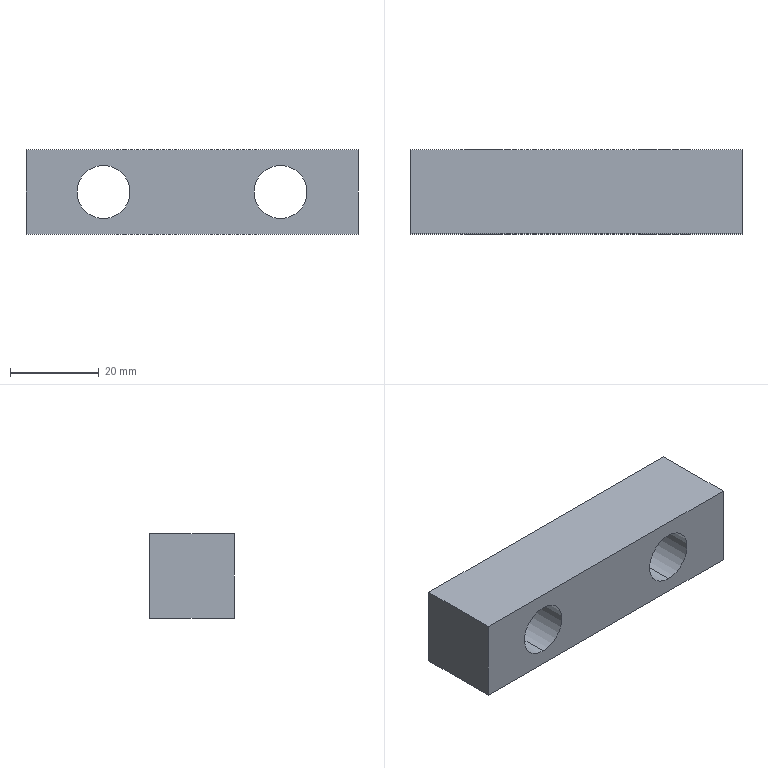Part | STEP file | [04]-1 | 1 solid | 10 faces | box 75 x 19 x 19 mm | volume 22777 mm3 | plane 6 | cylinder 4 | commonest cylinder face diameters 12 x4
STEP:
#1=CARTESIAN_POINT('',(0.,0.,0.));
#2=DIRECTION('',(0.,0.,1.));
#3=DIRECTION('',(1.,0.,0.));
#4=AXIS2_PLACEMENT_3D('',#1,#2,#3);
#5=CARTESIAN_POINT('',(17.5,-19.,15.5));
#6=VERTEX_POINT('',#5);
#7=CARTESIAN_POINT('',(17.5,0.,15.5));
#8=VERTEX_POINT('',#7);
#9=CARTESIAN_POINT('',(17.5,-19.,15.5));
#10=DIRECTION('',(0.,1.,0.));
#11=VECTOR('',#10,1.);
#12=LINE('',#9,#11);
#13=CARTESIAN_POINT('',(17.5,-19.,9.5));
#14=DIRECTION('',(0.,1.,0.));
#15=DIRECTION('',(0.,0.,1.));
#16=AXIS2_PLACEMENT_3D('',#13,#14,#15);
#17=CYLINDRICAL_SURFACE('',#16,6.);
#18=CARTESIAN_POINT('',(6.283,0.));
#19=DIRECTION('',(0.,1.));
#20=VECTOR('',#19,1.);
#21=LINE('',#18,#20);
#22=(GEOMETRIC_REPRESENTATION_CONTEXT(2)PARAMETRIC_REPRESENTATION_CONTEXT()REPRESENTATION_CONTEXT('',''));
#23=DEFINITIONAL_REPRESENTATION('',(#21),#22);
#24=PCURVE('',#17,#23);
#25=CARTESIAN_POINT('',(17.5,-19.,9.5));
#26=DIRECTION('',(0.,1.,0.));
#27=DIRECTION('',(0.,0.,1.));
#28=AXIS2_PLACEMENT_3D('',#25,#26,#27);
#29=CYLINDRICAL_SURFACE('',#28,6.);
#30=CARTESIAN_POINT('',(0.,0.));
#31=DIRECTION('',(0.,1.));
#32=VECTOR('',#31,1.);
#33=LINE('',#30,#32);
#34=(GEOMETRIC_REPRESENTATION_CONTEXT(2)PARAMETRIC_REPRESENTATION_CONTEXT()REPRESENTATION_CONTEXT('',''));
#35=DEFINITIONAL_REPRESENTATION('',(#33),#34);
#36=PCURVE('',#29,#35);
#37=SURFACE_CURVE('',#12,(#24,#36),.PCURVE_S1.);
#38=EDGE_CURVE('',#6,#8,#37,.T.);
#39=ORIENTED_EDGE('',*,*,#38,.T.);
#40=CARTESIAN_POINT('',(17.5,0.,3.5));
#41=VERTEX_POINT('',#40);
#42=CARTESIAN_POINT('',(17.5,0.,9.5));
#43=DIRECTION('',(0.,1.,0.));
#44=DIRECTION('',(0.,0.,-1.));
#45=AXIS2_PLACEMENT_3D('',#42,#43,#44);
#46=CIRCLE('',#45,6.);
#47=CARTESIAN_POINT('',(3.142,19.));
#48=DIRECTION('',(1.,0.));
#49=VECTOR('',#48,1.);
#50=LINE('',#47,#49);
#51=(GEOMETRIC_REPRESENTATION_CONTEXT(2)PARAMETRIC_REPRESENTATION_CONTEXT()REPRESENTATION_CONTEXT('',''));
#52=DEFINITIONAL_REPRESENTATION('',(#50),#51);
#53=PCURVE('',#17,#52);
#54=CARTESIAN_POINT('',(37.5,0.,0.));
#55=DIRECTION('',(0.,1.,0.));
#56=DIRECTION('',(0.,0.,1.));
#57=AXIS2_PLACEMENT_3D('',#54,#55,#56);
#58=PLANE('',#57);
#59=CARTESIAN_POINT('',(9.5,-20.));
#60=DIRECTION('',(-1.,0.));
#61=AXIS2_PLACEMENT_2D('',#59,#60);
#62=CIRCLE('',#61,6.);
#63=(GEOMETRIC_REPRESENTATION_CONTEXT(2)PARAMETRIC_REPRESENTATION_CONTEXT()REPRESENTATION_CONTEXT('',''));
#64=DEFINITIONAL_REPRESENTATION('',(#62),#63);
#65=PCURVE('',#58,#64);
#66=SURFACE_CURVE('',#46,(#53,#65),.PCURVE_S1.);
#67=EDGE_CURVE('',#41,#8,#66,.T.);
#68=ORIENTED_EDGE('',*,*,#67,.F.);
#69=CARTESIAN_POINT('',(17.5,-19.,3.5));
#70=VERTEX_POINT('',#69);
#71=CARTESIAN_POINT('',(17.5,-19.,3.5));
#72=DIRECTION('',(0.,1.,0.));
#73=VECTOR('',#72,1.);
#74=LINE('',#71,#73);
#75=CARTESIAN_POINT('',(3.142,0.));
#76=DIRECTION('',(0.,1.));
#77=VECTOR('',#76,1.);
#78=LINE('',#75,#77);
#79=(GEOMETRIC_REPRESENTATION_CONTEXT(2)PARAMETRIC_REPRESENTATION_CONTEXT()REPRESENTATION_CONTEXT('',''));
#80=DEFINITIONAL_REPRESENTATION('',(#78),#79);
#81=PCURVE('',#17,#80);
#82=CARTESIAN_POINT('',(3.142,0.));
#83=DIRECTION('',(0.,1.));
#84=VECTOR('',#83,1.);
#85=LINE('',#82,#84);
#86=(GEOMETRIC_REPRESENTATION_CONTEXT(2)PARAMETRIC_REPRESENTATION_CONTEXT()REPRESENTATION_CONTEXT('',''));
#87=DEFINITIONAL_REPRESENTATION('',(#85),#86);
#88=PCURVE('',#29,#87);
#89=SURFACE_CURVE('',#74,(#81,#88),.PCURVE_S1.);
#90=EDGE_CURVE('',#70,#41,#89,.T.);
#91=ORIENTED_EDGE('',*,*,#90,.F.);
#92=CARTESIAN_POINT('',(17.5,-19.,9.5));
#93=DIRECTION('',(0.,-1.,0.));
#94=DIRECTION('',(0.,0.,1.));
#95=AXIS2_PLACEMENT_3D('',#92,#93,#94);
#96=CIRCLE('',#95,6.);
#97=CARTESIAN_POINT('',(6.283,0.));
#98=DIRECTION('',(-1.,0.));
#99=VECTOR('',#98,1.);
#100=LINE('',#97,#99);
#101=(GEOMETRIC_REPRESENTATION_CONTEXT(2)PARAMETRIC_REPRESENTATION_CONTEXT()REPRESENTATION_CONTEXT('',''));
#102=DEFINITIONAL_REPRESENTATION('',(#100),#101);
#103=PCURVE('',#17,#102);
#104=CARTESIAN_POINT('',(37.5,-19.,0.));
#105=DIRECTION('',(0.,-1.,0.));
#106=DIRECTION('',(0.,0.,-1.));
#107=AXIS2_PLACEMENT_3D('',#104,#105,#106);
#108=PLANE('',#107);
#109=CARTESIAN_POINT('',(-9.5,-20.));
#110=DIRECTION('',(-1.,0.));
#111=AXIS2_PLACEMENT_2D('',#109,#110);
#112=CIRCLE('',#111,6.);
#113=(GEOMETRIC_REPRESENTATION_CONTEXT(2)PARAMETRIC_REPRESENTATION_CONTEXT()REPRESENTATION_CONTEXT('',''));
#114=DEFINITIONAL_REPRESENTATION('',(#112),#113);
#115=PCURVE('',#108,#114);
#116=SURFACE_CURVE('',#96,(#103,#115),.PCURVE_S1.);
#117=EDGE_CURVE('',#6,#70,#116,.T.);
#118=ORIENTED_EDGE('',*,*,#117,.F.);
#119=EDGE_LOOP('',(#39,#68,#91,#118));
#120=FACE_BOUND('',#119,.F.);
#121=ADVANCED_FACE('',(#120),#17,.F.);
#122=CARTESIAN_POINT('',(57.5,-19.,15.5));
#123=VERTEX_POINT('',#122);
#124=CARTESIAN_POINT('',(57.5,0.,15.5));
#125=VERTEX_POINT('',#124);
#126=CARTESIAN_POINT('',(57.5,-19.,15.5));
#127=DIRECTION('',(0.,1.,0.));
#128=VECTOR('',#127,1.);
#129=LINE('',#126,#128);
#130=CARTESIAN_POINT('',(57.5,-19.,9.5));
#131=DIRECTION('',(0.,1.,0.));
#132=DIRECTION('',(0.,0.,1.));
#133=AXIS2_PLACEMENT_3D('',#130,#131,#132);
#134=CYLINDRICAL_SURFACE('',#133,6.);
#135=CARTESIAN_POINT('',(6.283,0.));
#136=DIRECTION('',(0.,1.));
#137=VECTOR('',#136,1.);
#138=LINE('',#135,#137);
#139=(GEOMETRIC_REPRESENTATION_CONTEXT(2)PARAMETRIC_REPRESENTATION_CONTEXT()REPRESENTATION_CONTEXT('',''));
#140=DEFINITIONAL_REPRESENTATION('',(#138),#139);
#141=PCURVE('',#134,#140);
#142=CARTESIAN_POINT('',(57.5,-19.,9.5));
#143=DIRECTION('',(0.,1.,0.));
#144=DIRECTION('',(0.,0.,1.));
#145=AXIS2_PLACEMENT_3D('',#142,#143,#144);
#146=CYLINDRICAL_SURFACE('',#145,6.);
#147=CARTESIAN_POINT('',(0.,0.));
#148=DIRECTION('',(0.,1.));
#149=VECTOR('',#148,1.);
#150=LINE('',#147,#149);
#151=(GEOMETRIC_REPRESENTATION_CONTEXT(2)PARAMETRIC_REPRESENTATION_CONTEXT()REPRESENTATION_CONTEXT('',''));
#152=DEFINITIONAL_REPRESENTATION('',(#150),#151);
#153=PCURVE('',#146,#152);
#154=SURFACE_CURVE('',#129,(#141,#153),.PCURVE_S1.);
#155=EDGE_CURVE('',#123,#125,#154,.T.);
#156=ORIENTED_EDGE('',*,*,#155,.T.);
#157=CARTESIAN_POINT('',(57.5,0.,3.5));
#158=VERTEX_POINT('',#157);
#159=CARTESIAN_POINT('',(57.5,0.,9.5));
#160=DIRECTION('',(0.,1.,0.));
#161=DIRECTION('',(0.,0.,-1.));
#162=AXIS2_PLACEMENT_3D('',#159,#160,#161);
#163=CIRCLE('',#162,6.);
#164=CARTESIAN_POINT('',(3.142,19.));
#165=DIRECTION('',(1.,0.));
#166=VECTOR('',#165,1.);
#167=LINE('',#164,#166);
#168=(GEOMETRIC_REPRESENTATION_CONTEXT(2)PARAMETRIC_REPRESENTATION_CONTEXT()REPRESENTATION_CONTEXT('',''));
#169=DEFINITIONAL_REPRESENTATION('',(#167),#168);
#170=PCURVE('',#134,#169);
#171=CARTESIAN_POINT('',(9.5,20.));
#172=DIRECTION('',(-1.,0.));
#173=AXIS2_PLACEMENT_2D('',#171,#172);
#174=CIRCLE('',#173,6.);
#175=(GEOMETRIC_REPRESENTATION_CONTEXT(2)PARAMETRIC_REPRESENTATION_CONTEXT()REPRESENTATION_CONTEXT('',''));
#176=DEFINITIONAL_REPRESENTATION('',(#174),#175);
#177=PCURVE('',#58,#176);
#178=SURFACE_CURVE('',#163,(#170,#177),.PCURVE_S1.);
#179=EDGE_CURVE('',#158,#125,#178,.T.);
#180=ORIENTED_EDGE('',*,*,#179,.F.);
#181=CARTESIAN_POINT('',(57.5,-19.,3.5));
#182=VERTEX_POINT('',#181);
#183=CARTESIAN_POINT('',(57.5,-19.,3.5));
#184=DIRECTION('',(0.,1.,0.));
#185=VECTOR('',#184,1.);
#186=LINE('',#183,#185);
#187=CARTESIAN_POINT('',(3.142,0.));
#188=DIRECTION('',(0.,1.));
#189=VECTOR('',#188,1.);
#190=LINE('',#187,#189);
#191=(GEOMETRIC_REPRESENTATION_CONTEXT(2)PARAMETRIC_REPRESENTATION_CONTEXT()REPRESENTATION_CONTEXT('',''));
#192=DEFINITIONAL_REPRESENTATION('',(#190),#191);
#193=PCURVE('',#134,#192);
#194=CARTESIAN_POINT('',(3.142,0.));
#195=DIRECTION('',(0.,1.));
#196=VECTOR('',#195,1.);
#197=LINE('',#194,#196);
#198=(GEOMETRIC_REPRESENTATION_CONTEXT(2)PARAMETRIC_REPRESENTATION_CONTEXT()REPRESENTATION_CONTEXT('',''));
#199=DEFINITIONAL_REPRESENTATION('',(#197),#198);
#200=PCURVE('',#146,#199);
#201=SURFACE_CURVE('',#186,(#193,#200),.PCURVE_S1.);
#202=EDGE_CURVE('',#182,#158,#201,.T.);
#203=ORIENTED_EDGE('',*,*,#202,.F.);
#204=CARTESIAN_POINT('',(57.5,-19.,9.5));
#205=DIRECTION('',(0.,-1.,0.));
#206=DIRECTION('',(0.,0.,1.));
#207=AXIS2_PLACEMENT_3D('',#204,#205,#206);
#208=CIRCLE('',#207,6.);
#209=CARTESIAN_POINT('',(6.283,0.));
#210=DIRECTION('',(-1.,0.));
#211=VECTOR('',#210,1.);
#212=LINE('',#209,#211);
#213=(GEOMETRIC_REPRESENTATION_CONTEXT(2)PARAMETRIC_REPRESENTATION_CONTEXT()REPRESENTATION_CONTEXT('',''));
#214=DEFINITIONAL_REPRESENTATION('',(#212),#213);
#215=PCURVE('',#134,#214);
#216=CARTESIAN_POINT('',(-9.5,20.));
#217=DIRECTION('',(-1.,0.));
#218=AXIS2_PLACEMENT_2D('',#216,#217);
#219=CIRCLE('',#218,6.);
#220=(GEOMETRIC_REPRESENTATION_CONTEXT(2)PARAMETRIC_REPRESENTATION_CONTEXT()REPRESENTATION_CONTEXT('',''));
#221=DEFINITIONAL_REPRESENTATION('',(#219),#220);
#222=PCURVE('',#108,#221);
#223=SURFACE_CURVE('',#208,(#215,#222),.PCURVE_S1.);
#224=EDGE_CURVE('',#123,#182,#223,.T.);
#225=ORIENTED_EDGE('',*,*,#224,.F.);
#226=EDGE_LOOP('',(#156,#180,#203,#225));
#227=FACE_BOUND('',#226,.F.);
#228=ADVANCED_FACE('',(#227),#134,.F.);
#229=CARTESIAN_POINT('',(0.,-19.,19.));
#230=VERTEX_POINT('',#229);
#231=CARTESIAN_POINT('',(75.,-19.,19.));
#232=VERTEX_POINT('',#231);
#233=CARTESIAN_POINT('',(37.5,-19.,19.));
#234=DIRECTION('',(1.,0.,0.));
#235=VECTOR('',#234,1.);
#236=LINE('',#233,#235);
#237=CARTESIAN_POINT('',(37.5,-9.5,19.));
#238=DIRECTION('',(0.,0.,1.));
#239=DIRECTION('',(-1.,0.,0.));
#240=AXIS2_PLACEMENT_3D('',#237,#238,#239);
#241=PLANE('',#240);
#242=CARTESIAN_POINT('',(0.,9.5));
#243=DIRECTION('',(-1.,0.));
#244=VECTOR('',#243,1.);
#245=LINE('',#242,#244);
#246=(GEOMETRIC_REPRESENTATION_CONTEXT(2)PARAMETRIC_REPRESENTATION_CONTEXT()REPRESENTATION_CONTEXT('',''));
#247=DEFINITIONAL_REPRESENTATION('',(#245),#246);
#248=PCURVE('',#241,#247);
#249=CARTESIAN_POINT('',(-19.,0.));
#250=DIRECTION('',(0.,1.));
#251=VECTOR('',#250,1.);
#252=LINE('',#249,#251);
#253=(GEOMETRIC_REPRESENTATION_CONTEXT(2)PARAMETRIC_REPRESENTATION_CONTEXT()REPRESENTATION_CONTEXT('',''));
#254=DEFINITIONAL_REPRESENTATION('',(#252),#253);
#255=PCURVE('',#108,#254);
#256=SURFACE_CURVE('',#236,(#248,#255),.PCURVE_S1.);
#257=EDGE_CURVE('',#230,#232,#256,.T.);
#258=ORIENTED_EDGE('',*,*,#257,.T.);
#259=CARTESIAN_POINT('',(75.,0.,19.));
#260=VERTEX_POINT('',#259);
#261=CARTESIAN_POINT('',(75.,-9.5,19.));
#262=DIRECTION('',(0.,1.,0.));
#263=VECTOR('',#262,1.);
#264=LINE('',#261,#263);
#265=CARTESIAN_POINT('',(-37.5,0.));
#266=DIRECTION('',(0.,-1.));
#267=VECTOR('',#266,1.);
#268=LINE('',#265,#267);
#269=(GEOMETRIC_REPRESENTATION_CONTEXT(2)PARAMETRIC_REPRESENTATION_CONTEXT()REPRESENTATION_CONTEXT('',''));
#270=DEFINITIONAL_REPRESENTATION('',(#268),#269);
#271=PCURVE('',#241,#270);
#272=CARTESIAN_POINT('',(75.,-9.5,0.));
#273=DIRECTION('',(1.,0.,0.));
#274=DIRECTION('',(0.,0.,1.));
#275=AXIS2_PLACEMENT_3D('',#272,#273,#274);
#276=PLANE('',#275);
#277=CARTESIAN_POINT('',(19.,0.));
#278=DIRECTION('',(0.,-1.));
#279=VECTOR('',#278,1.);
#280=LINE('',#277,#279);
#281=(GEOMETRIC_REPRESENTATION_CONTEXT(2)PARAMETRIC_REPRESENTATION_CONTEXT()REPRESENTATION_CONTEXT('',''));
#282=DEFINITIONAL_REPRESENTATION('',(#280),#281);
#283=PCURVE('',#276,#282);
#284=SURFACE_CURVE('',#264,(#271,#283),.PCURVE_S1.);
#285=EDGE_CURVE('',#232,#260,#284,.T.);
#286=ORIENTED_EDGE('',*,*,#285,.T.);
#287=CARTESIAN_POINT('',(0.,0.,19.));
#288=VERTEX_POINT('',#287);
#289=CARTESIAN_POINT('',(37.5,0.,19.));
#290=DIRECTION('',(-1.,0.,0.));
#291=VECTOR('',#290,1.);
#292=LINE('',#289,#291);
#293=CARTESIAN_POINT('',(0.,-9.5));
#294=DIRECTION('',(1.,0.));
#295=VECTOR('',#294,1.);
#296=LINE('',#293,#295);
#297=(GEOMETRIC_REPRESENTATION_CONTEXT(2)PARAMETRIC_REPRESENTATION_CONTEXT()REPRESENTATION_CONTEXT('',''));
#298=DEFINITIONAL_REPRESENTATION('',(#296),#297);
#299=PCURVE('',#241,#298);
#300=CARTESIAN_POINT('',(19.,0.));
#301=DIRECTION('',(0.,-1.));
#302=VECTOR('',#301,1.);
#303=LINE('',#300,#302);
#304=(GEOMETRIC_REPRESENTATION_CONTEXT(2)PARAMETRIC_REPRESENTATION_CONTEXT()REPRESENTATION_CONTEXT('',''));
#305=DEFINITIONAL_REPRESENTATION('',(#303),#304);
#306=PCURVE('',#58,#305);
#307=SURFACE_CURVE('',#292,(#299,#306),.PCURVE_S1.);
#308=EDGE_CURVE('',#260,#288,#307,.T.);
#309=ORIENTED_EDGE('',*,*,#308,.T.);
#310=CARTESIAN_POINT('',(0.,-9.5,19.));
#311=DIRECTION('',(0.,-1.,0.));
#312=VECTOR('',#311,1.);
#313=LINE('',#310,#312);
#314=CARTESIAN_POINT('',(37.5,0.));
#315=DIRECTION('',(0.,1.));
#316=VECTOR('',#315,1.);
#317=LINE('',#314,#316);
#318=(GEOMETRIC_REPRESENTATION_CONTEXT(2)PARAMETRIC_REPRESENTATION_CONTEXT()REPRESENTATION_CONTEXT('',''));
#319=DEFINITIONAL_REPRESENTATION('',(#317),#318);
#320=PCURVE('',#241,#319);
#321=CARTESIAN_POINT('',(0.,-9.5,0.));
#322=DIRECTION('',(-1.,0.,0.));
#323=DIRECTION('',(0.,0.,-1.));
#324=AXIS2_PLACEMENT_3D('',#321,#322,#323);
#325=PLANE('',#324);
#326=CARTESIAN_POINT('',(-19.,0.));
#327=DIRECTION('',(0.,1.));
#328=VECTOR('',#327,1.);
#329=LINE('',#326,#328);
#330=(GEOMETRIC_REPRESENTATION_CONTEXT(2)PARAMETRIC_REPRESENTATION_CONTEXT()REPRESENTATION_CONTEXT('',''));
#331=DEFINITIONAL_REPRESENTATION('',(#329),#330);
#332=PCURVE('',#325,#331);
#333=SURFACE_CURVE('',#313,(#320,#332),.PCURVE_S1.);
#334=EDGE_CURVE('',#288,#230,#333,.T.);
#335=ORIENTED_EDGE('',*,*,#334,.T.);
#336=EDGE_LOOP('',(#258,#286,#309,#335));
#337=FACE_BOUND('',#336,.T.);
#338=ADVANCED_FACE('',(#337),#241,.T.);
#339=ORIENTED_EDGE('',*,*,#117,.F.);
#340=CARTESIAN_POINT('',(17.5,-19.,9.5));
#341=DIRECTION('',(0.,-1.,0.));
#342=DIRECTION('',(0.,0.,1.));
#343=AXIS2_PLACEMENT_3D('',#340,#341,#342);
#344=CIRCLE('',#343,6.);
#345=CARTESIAN_POINT('',(-9.5,-20.));
#346=DIRECTION('',(-1.,0.));
#347=AXIS2_PLACEMENT_2D('',#345,#346);
#348=CIRCLE('',#347,6.);
#349=(GEOMETRIC_REPRESENTATION_CONTEXT(2)PARAMETRIC_REPRESENTATION_CONTEXT()REPRESENTATION_CONTEXT('',''));
#350=DEFINITIONAL_REPRESENTATION('',(#348),#349);
#351=PCURVE('',#108,#350);
#352=CARTESIAN_POINT('',(6.283,0.));
#353=DIRECTION('',(-1.,0.));
#354=VECTOR('',#353,1.);
#355=LINE('',#352,#354);
#356=(GEOMETRIC_REPRESENTATION_CONTEXT(2)PARAMETRIC_REPRESENTATION_CONTEXT()REPRESENTATION_CONTEXT('',''));
#357=DEFINITIONAL_REPRESENTATION('',(#355),#356);
#358=PCURVE('',#29,#357);
#359=SURFACE_CURVE('',#344,(#351,#358),.PCURVE_S1.);
#360=EDGE_CURVE('',#70,#6,#359,.T.);
#361=ORIENTED_EDGE('',*,*,#360,.F.);
#362=EDGE_LOOP('',(#339,#361));
#363=FACE_BOUND('',#362,.T.);
#364=ORIENTED_EDGE('',*,*,#224,.F.);
#365=CARTESIAN_POINT('',(57.5,-19.,9.5));
#366=DIRECTION('',(0.,-1.,0.));
#367=DIRECTION('',(0.,0.,1.));
#368=AXIS2_PLACEMENT_3D('',#365,#366,#367);
#369=CIRCLE('',#368,6.);
#370=CARTESIAN_POINT('',(-9.5,20.));
#371=DIRECTION('',(-1.,0.));
#372=AXIS2_PLACEMENT_2D('',#370,#371);
#373=CIRCLE('',#372,6.);
#374=(GEOMETRIC_REPRESENTATION_CONTEXT(2)PARAMETRIC_REPRESENTATION_CONTEXT()REPRESENTATION_CONTEXT('',''));
#375=DEFINITIONAL_REPRESENTATION('',(#373),#374);
#376=PCURVE('',#108,#375);
#377=CARTESIAN_POINT('',(6.283,0.));
#378=DIRECTION('',(-1.,0.));
#379=VECTOR('',#378,1.);
#380=LINE('',#377,#379);
#381=(GEOMETRIC_REPRESENTATION_CONTEXT(2)PARAMETRIC_REPRESENTATION_CONTEXT()REPRESENTATION_CONTEXT('',''));
#382=DEFINITIONAL_REPRESENTATION('',(#380),#381);
#383=PCURVE('',#146,#382);
#384=SURFACE_CURVE('',#369,(#376,#383),.PCURVE_S1.);
#385=EDGE_CURVE('',#182,#123,#384,.T.);
#386=ORIENTED_EDGE('',*,*,#385,.F.);
#387=EDGE_LOOP('',(#364,#386));
#388=FACE_BOUND('',#387,.T.);
#389=CARTESIAN_POINT('',(0.,-19.,0.));
#390=VERTEX_POINT('',#389);
#391=CARTESIAN_POINT('',(0.,-19.,0.));
#392=DIRECTION('',(0.,0.,1.));
#393=VECTOR('',#392,1.);
#394=LINE('',#391,#393);
#395=CARTESIAN_POINT('',(0.,-37.5));
#396=DIRECTION('',(-1.,0.));
#397=VECTOR('',#396,1.);
#398=LINE('',#395,#397);
#399=(GEOMETRIC_REPRESENTATION_CONTEXT(2)PARAMETRIC_REPRESENTATION_CONTEXT()REPRESENTATION_CONTEXT('',''));
#400=DEFINITIONAL_REPRESENTATION('',(#398),#399);
#401=PCURVE('',#108,#400);
#402=CARTESIAN_POINT('',(0.,9.5));
#403=DIRECTION('',(-1.,0.));
#404=VECTOR('',#403,1.);
#405=LINE('',#402,#404);
#406=(GEOMETRIC_REPRESENTATION_CONTEXT(2)PARAMETRIC_REPRESENTATION_CONTEXT()REPRESENTATION_CONTEXT('',''));
#407=DEFINITIONAL_REPRESENTATION('',(#405),#406);
#408=PCURVE('',#325,#407);
#409=SURFACE_CURVE('',#394,(#401,#408),.PCURVE_S1.);
#410=EDGE_CURVE('',#390,#230,#409,.T.);
#411=ORIENTED_EDGE('',*,*,#410,.F.);
#412=CARTESIAN_POINT('',(75.,-19.,0.));
#413=VERTEX_POINT('',#412);
#414=CARTESIAN_POINT('',(37.5,-19.,0.));
#415=DIRECTION('',(-1.,0.,0.));
#416=VECTOR('',#415,1.);
#417=LINE('',#414,#416);
#418=CARTESIAN_POINT('',(0.,0.));
#419=DIRECTION('',(0.,-1.));
#420=VECTOR('',#419,1.);
#421=LINE('',#418,#420);
#422=(GEOMETRIC_REPRESENTATION_CONTEXT(2)PARAMETRIC_REPRESENTATION_CONTEXT()REPRESENTATION_CONTEXT('',''));
#423=DEFINITIONAL_REPRESENTATION('',(#421),#422);
#424=PCURVE('',#108,#423);
#425=CARTESIAN_POINT('',(37.5,-9.5,0.));
#426=DIRECTION('',(0.,0.,-1.));
#427=DIRECTION('',(1.,0.,0.));
#428=AXIS2_PLACEMENT_3D('',#425,#426,#427);
#429=PLANE('',#428);
#430=CARTESIAN_POINT('',(0.,9.5));
#431=DIRECTION('',(-1.,0.));
#432=VECTOR('',#431,1.);
#433=LINE('',#430,#432);
#434=(GEOMETRIC_REPRESENTATION_CONTEXT(2)PARAMETRIC_REPRESENTATION_CONTEXT()REPRESENTATION_CONTEXT('',''));
#435=DEFINITIONAL_REPRESENTATION('',(#433),#434);
#436=PCURVE('',#429,#435);
#437=SURFACE_CURVE('',#417,(#424,#436),.PCURVE_S1.);
#438=EDGE_CURVE('',#413,#390,#437,.T.);
#439=ORIENTED_EDGE('',*,*,#438,.F.);
#440=CARTESIAN_POINT('',(75.,-19.,0.));
#441=DIRECTION('',(0.,0.,1.));
#442=VECTOR('',#441,1.);
#443=LINE('',#440,#442);
#444=CARTESIAN_POINT('',(0.,37.5));
#445=DIRECTION('',(-1.,0.));
#446=VECTOR('',#445,1.);
#447=LINE('',#444,#446);
#448=(GEOMETRIC_REPRESENTATION_CONTEXT(2)PARAMETRIC_REPRESENTATION_CONTEXT()REPRESENTATION_CONTEXT('',''));
#449=DEFINITIONAL_REPRESENTATION('',(#447),#448);
#450=PCURVE('',#108,#449);
#451=CARTESIAN_POINT('',(0.,9.5));
#452=DIRECTION('',(1.,0.));
#453=VECTOR('',#452,1.);
#454=LINE('',#451,#453);
#455=(GEOMETRIC_REPRESENTATION_CONTEXT(2)PARAMETRIC_REPRESENTATION_CONTEXT()REPRESENTATION_CONTEXT('',''));
#456=DEFINITIONAL_REPRESENTATION('',(#454),#455);
#457=PCURVE('',#276,#456);
#458=SURFACE_CURVE('',#443,(#450,#457),.PCURVE_S1.);
#459=EDGE_CURVE('',#413,#232,#458,.T.);
#460=ORIENTED_EDGE('',*,*,#459,.T.);
#461=ORIENTED_EDGE('',*,*,#257,.F.);
#462=EDGE_LOOP('',(#411,#439,#460,#461));
#463=FACE_BOUND('',#462,.T.);
#464=ADVANCED_FACE('',(#363,#388,#463),#108,.T.);
#465=ORIENTED_EDGE('',*,*,#459,.F.);
#466=CARTESIAN_POINT('',(75.,0.,0.));
#467=VERTEX_POINT('',#466);
#468=CARTESIAN_POINT('',(75.,-9.5,0.));
#469=DIRECTION('',(0.,-1.,0.));
#470=VECTOR('',#469,1.);
#471=LINE('',#468,#470);
#472=CARTESIAN_POINT('',(0.,0.));
#473=DIRECTION('',(0.,1.));
#474=VECTOR('',#473,1.);
#475=LINE('',#472,#474);
#476=(GEOMETRIC_REPRESENTATION_CONTEXT(2)PARAMETRIC_REPRESENTATION_CONTEXT()REPRESENTATION_CONTEXT('',''));
#477=DEFINITIONAL_REPRESENTATION('',(#475),#476);
#478=PCURVE('',#276,#477);
#479=CARTESIAN_POINT('',(37.5,0.));
#480=DIRECTION('',(0.,1.));
#481=VECTOR('',#480,1.);
#482=LINE('',#479,#481);
#483=(GEOMETRIC_REPRESENTATION_CONTEXT(2)PARAMETRIC_REPRESENTATION_CONTEXT()REPRESENTATION_CONTEXT('',''));
#484=DEFINITIONAL_REPRESENTATION('',(#482),#483);
#485=PCURVE('',#429,#484);
#486=SURFACE_CURVE('',#471,(#478,#485),.PCURVE_S1.);
#487=EDGE_CURVE('',#467,#413,#486,.T.);
#488=ORIENTED_EDGE('',*,*,#487,.F.);
#489=CARTESIAN_POINT('',(75.,0.,0.));
#490=DIRECTION('',(0.,0.,1.));
#491=VECTOR('',#490,1.);
#492=LINE('',#489,#491);
#493=CARTESIAN_POINT('',(0.,-9.5));
#494=DIRECTION('',(1.,0.));
#495=VECTOR('',#494,1.);
#496=LINE('',#493,#495);
#497=(GEOMETRIC_REPRESENTATION_CONTEXT(2)PARAMETRIC_REPRESENTATION_CONTEXT()REPRESENTATION_CONTEXT('',''));
#498=DEFINITIONAL_REPRESENTATION('',(#496),#497);
#499=PCURVE('',#276,#498);
#500=CARTESIAN_POINT('',(0.,37.5));
#501=DIRECTION('',(1.,0.));
#502=VECTOR('',#501,1.);
#503=LINE('',#500,#502);
#504=(GEOMETRIC_REPRESENTATION_CONTEXT(2)PARAMETRIC_REPRESENTATION_CONTEXT()REPRESENTATION_CONTEXT('',''));
#505=DEFINITIONAL_REPRESENTATION('',(#503),#504);
#506=PCURVE('',#58,#505);
#507=SURFACE_CURVE('',#492,(#499,#506),.PCURVE_S1.);
#508=EDGE_CURVE('',#467,#260,#507,.T.);
#509=ORIENTED_EDGE('',*,*,#508,.T.);
#510=ORIENTED_EDGE('',*,*,#285,.F.);
#511=EDGE_LOOP('',(#465,#488,#509,#510));
#512=FACE_BOUND('',#511,.T.);
#513=ADVANCED_FACE('',(#512),#276,.T.);
#514=CARTESIAN_POINT('',(17.5,0.,9.5));
#515=DIRECTION('',(0.,1.,0.));
#516=DIRECTION('',(0.,0.,-1.));
#517=AXIS2_PLACEMENT_3D('',#514,#515,#516);
#518=CIRCLE('',#517,6.);
#519=CARTESIAN_POINT('',(9.5,-20.));
#520=DIRECTION('',(-1.,0.));
#521=AXIS2_PLACEMENT_2D('',#519,#520);
#522=CIRCLE('',#521,6.);
#523=(GEOMETRIC_REPRESENTATION_CONTEXT(2)PARAMETRIC_REPRESENTATION_CONTEXT()REPRESENTATION_CONTEXT('',''));
#524=DEFINITIONAL_REPRESENTATION('',(#522),#523);
#525=PCURVE('',#58,#524);
#526=CARTESIAN_POINT('',(-3.142,19.));
#527=DIRECTION('',(1.,0.));
#528=VECTOR('',#527,1.);
#529=LINE('',#526,#528);
#530=(GEOMETRIC_REPRESENTATION_CONTEXT(2)PARAMETRIC_REPRESENTATION_CONTEXT()REPRESENTATION_CONTEXT('',''));
#531=DEFINITIONAL_REPRESENTATION('',(#529),#530);
#532=PCURVE('',#29,#531);
#533=SURFACE_CURVE('',#518,(#525,#532),.PCURVE_S1.);
#534=EDGE_CURVE('',#8,#41,#533,.T.);
#535=ORIENTED_EDGE('',*,*,#534,.F.);
#536=ORIENTED_EDGE('',*,*,#67,.F.);
#537=EDGE_LOOP('',(#535,#536));
#538=FACE_BOUND('',#537,.T.);
#539=CARTESIAN_POINT('',(57.5,0.,9.5));
#540=DIRECTION('',(0.,1.,0.));
#541=DIRECTION('',(0.,0.,-1.));
#542=AXIS2_PLACEMENT_3D('',#539,#540,#541);
#543=CIRCLE('',#542,6.);
#544=CARTESIAN_POINT('',(9.5,20.));
#545=DIRECTION('',(-1.,0.));
#546=AXIS2_PLACEMENT_2D('',#544,#545);
#547=CIRCLE('',#546,6.);
#548=(GEOMETRIC_REPRESENTATION_CONTEXT(2)PARAMETRIC_REPRESENTATION_CONTEXT()REPRESENTATION_CONTEXT('',''));
#549=DEFINITIONAL_REPRESENTATION('',(#547),#548);
#550=PCURVE('',#58,#549);
#551=CARTESIAN_POINT('',(-3.142,19.));
#552=DIRECTION('',(1.,0.));
#553=VECTOR('',#552,1.);
#554=LINE('',#551,#553);
#555=(GEOMETRIC_REPRESENTATION_CONTEXT(2)PARAMETRIC_REPRESENTATION_CONTEXT()REPRESENTATION_CONTEXT('',''));
#556=DEFINITIONAL_REPRESENTATION('',(#554),#555);
#557=PCURVE('',#146,#556);
#558=SURFACE_CURVE('',#543,(#550,#557),.PCURVE_S1.);
#559=EDGE_CURVE('',#125,#158,#558,.T.);
#560=ORIENTED_EDGE('',*,*,#559,.F.);
#561=ORIENTED_EDGE('',*,*,#179,.F.);
#562=EDGE_LOOP('',(#560,#561));
#563=FACE_BOUND('',#562,.T.);
#564=ORIENTED_EDGE('',*,*,#508,.F.);
#565=CARTESIAN_POINT('',(0.,0.,0.));
#566=VERTEX_POINT('',#565);
#567=CARTESIAN_POINT('',(37.5,0.,0.));
#568=DIRECTION('',(1.,0.,0.));
#569=VECTOR('',#568,1.);
#570=LINE('',#567,#569);
#571=CARTESIAN_POINT('',(0.,0.));
#572=DIRECTION('',(0.,1.));
#573=VECTOR('',#572,1.);
#574=LINE('',#571,#573);
#575=(GEOMETRIC_REPRESENTATION_CONTEXT(2)PARAMETRIC_REPRESENTATION_CONTEXT()REPRESENTATION_CONTEXT('',''));
#576=DEFINITIONAL_REPRESENTATION('',(#574),#575);
#577=PCURVE('',#58,#576);
#578=CARTESIAN_POINT('',(0.,-9.5));
#579=DIRECTION('',(1.,0.));
#580=VECTOR('',#579,1.);
#581=LINE('',#578,#580);
#582=(GEOMETRIC_REPRESENTATION_CONTEXT(2)PARAMETRIC_REPRESENTATION_CONTEXT()REPRESENTATION_CONTEXT('',''));
#583=DEFINITIONAL_REPRESENTATION('',(#581),#582);
#584=PCURVE('',#429,#583);
#585=SURFACE_CURVE('',#570,(#577,#584),.PCURVE_S1.);
#586=EDGE_CURVE('',#566,#467,#585,.T.);
#587=ORIENTED_EDGE('',*,*,#586,.F.);
#588=CARTESIAN_POINT('',(0.,0.,0.));
#589=DIRECTION('',(0.,0.,1.));
#590=VECTOR('',#589,1.);
#591=LINE('',#588,#590);
#592=CARTESIAN_POINT('',(0.,-37.5));
#593=DIRECTION('',(1.,0.));
#594=VECTOR('',#593,1.);
#595=LINE('',#592,#594);
#596=(GEOMETRIC_REPRESENTATION_CONTEXT(2)PARAMETRIC_REPRESENTATION_CONTEXT()REPRESENTATION_CONTEXT('',''));
#597=DEFINITIONAL_REPRESENTATION('',(#595),#596);
#598=PCURVE('',#58,#597);
#599=CARTESIAN_POINT('',(0.,-9.5));
#600=DIRECTION('',(-1.,0.));
#601=VECTOR('',#600,1.);
#602=LINE('',#599,#601);
#603=(GEOMETRIC_REPRESENTATION_CONTEXT(2)PARAMETRIC_REPRESENTATION_CONTEXT()REPRESENTATION_CONTEXT('',''));
#604=DEFINITIONAL_REPRESENTATION('',(#602),#603);
#605=PCURVE('',#325,#604);
#606=SURFACE_CURVE('',#591,(#598,#605),.PCURVE_S1.);
#607=EDGE_CURVE('',#566,#288,#606,.T.);
#608=ORIENTED_EDGE('',*,*,#607,.T.);
#609=ORIENTED_EDGE('',*,*,#308,.F.);
#610=EDGE_LOOP('',(#564,#587,#608,#609));
#611=FACE_BOUND('',#610,.T.);
#612=ADVANCED_FACE('',(#538,#563,#611),#58,.T.);
#613=CARTESIAN_POINT('',(0.,-9.5,0.));
#614=DIRECTION('',(0.,1.,0.));
#615=VECTOR('',#614,1.);
#616=LINE('',#613,#615);
#617=CARTESIAN_POINT('',(-37.5,0.));
#618=DIRECTION('',(0.,-1.));
#619=VECTOR('',#618,1.);
#620=LINE('',#617,#619);
#621=(GEOMETRIC_REPRESENTATION_CONTEXT(2)PARAMETRIC_REPRESENTATION_CONTEXT()REPRESENTATION_CONTEXT('',''));
#622=DEFINITIONAL_REPRESENTATION('',(#620),#621);
#623=PCURVE('',#429,#622);
#624=CARTESIAN_POINT('',(0.,0.));
#625=DIRECTION('',(0.,-1.));
#626=VECTOR('',#625,1.);
#627=LINE('',#624,#626);
#628=(GEOMETRIC_REPRESENTATION_CONTEXT(2)PARAMETRIC_REPRESENTATION_CONTEXT()REPRESENTATION_CONTEXT('',''));
#629=DEFINITIONAL_REPRESENTATION('',(#627),#628);
#630=PCURVE('',#325,#629);
#631=SURFACE_CURVE('',#616,(#623,#630),.PCURVE_S1.);
#632=EDGE_CURVE('',#390,#566,#631,.T.);
#633=ORIENTED_EDGE('',*,*,#632,.T.);
#634=ORIENTED_EDGE('',*,*,#586,.T.);
#635=ORIENTED_EDGE('',*,*,#487,.T.);
#636=ORIENTED_EDGE('',*,*,#438,.T.);
#637=EDGE_LOOP('',(#633,#634,#635,#636));
#638=FACE_BOUND('',#637,.T.);
#639=ADVANCED_FACE('',(#638),#429,.T.);
#640=ORIENTED_EDGE('',*,*,#632,.F.);
#641=ORIENTED_EDGE('',*,*,#410,.T.);
#642=ORIENTED_EDGE('',*,*,#334,.F.);
#643=ORIENTED_EDGE('',*,*,#607,.F.);
#644=EDGE_LOOP('',(#640,#641,#642,#643));
#645=FACE_BOUND('',#644,.T.);
#646=ADVANCED_FACE('',(#645),#325,.T.);
#647=ORIENTED_EDGE('',*,*,#559,.F.);
#648=ORIENTED_EDGE('',*,*,#155,.F.);
#649=ORIENTED_EDGE('',*,*,#385,.F.);
#650=ORIENTED_EDGE('',*,*,#202,.T.);
#651=EDGE_LOOP('',(#647,#648,#649,#650));
#652=FACE_BOUND('',#651,.F.);
#653=ADVANCED_FACE('',(#652),#146,.F.);
#654=ORIENTED_EDGE('',*,*,#534,.F.);
#655=ORIENTED_EDGE('',*,*,#38,.F.);
#656=ORIENTED_EDGE('',*,*,#360,.F.);
#657=ORIENTED_EDGE('',*,*,#90,.T.);
#658=EDGE_LOOP('',(#654,#655,#656,#657));
#659=FACE_BOUND('',#658,.F.);
#660=ADVANCED_FACE('',(#659),#29,.F.);
#661=CLOSED_SHELL('',(#121,#228,#338,#464,#513,#612,#639,#646,#653,#660));
#662=MANIFOLD_SOLID_BREP('',#661);
#663=(LENGTH_UNIT()NAMED_UNIT(*)SI_UNIT(.MILLI.,.METRE.));
#664=UNCERTAINTY_MEASURE_WITH_UNIT(LENGTH_MEASURE(0.0000001),#663,'','');
#665=(NAMED_UNIT(*)PLANE_ANGLE_UNIT()SI_UNIT($,.RADIAN.));
#666=(NAMED_UNIT(*)SI_UNIT($,.STERADIAN.)SOLID_ANGLE_UNIT());
#667=(GEOMETRIC_REPRESENTATION_CONTEXT(3)GLOBAL_UNCERTAINTY_ASSIGNED_CONTEXT((#664))GLOBAL_UNIT_ASSIGNED_CONTEXT((#663,#665,#666))REPRESENTATION_CONTEXT('',''));
#668=ADVANCED_BREP_SHAPE_REPRESENTATION('',(#4,#662),#667);